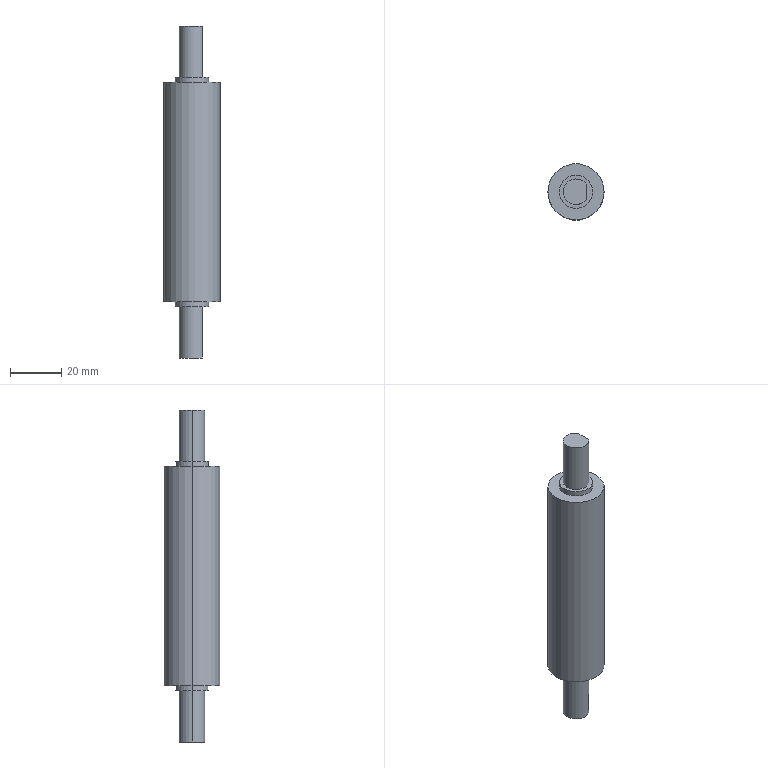Part | STEP file | 08-05 driven shaft | 1 solid | 18 faces | box 22 x 22 x 130 mm | volume 36200 mm3 | cylinder 10 | plane 8 | commonest cylinder face diameters 10 x4 13 x4 22 x2
STEP:
#1=CARTESIAN_POINT('',(-5.,0.,130.));
#2=VERTEX_POINT('',#1);
#3=CARTESIAN_POINT('',(4.,-3.,130.));
#4=VERTEX_POINT('',#3);
#5=CARTESIAN_POINT('',(0.,0.,130.));
#6=DIRECTION('',(0.,0.,1.));
#7=DIRECTION('',(1.,0.,0.));
#8=AXIS2_PLACEMENT_3D('',#5,#6,#7);
#9=CIRCLE('',#8,5.);
#10=EDGE_CURVE('',#2,#4,#9,.T.);
#11=ORIENTED_EDGE('',*,*,#10,.F.);
#12=CARTESIAN_POINT('',(-5.,0.,110.));
#13=VERTEX_POINT('',#12);
#14=CARTESIAN_POINT('',(-5.,0.,130.));
#15=DIRECTION('',(0.,0.,-1.));
#16=VECTOR('',#15,1000.);
#17=LINE('',#14,#16);
#18=EDGE_CURVE('',#2,#13,#17,.T.);
#19=ORIENTED_EDGE('',*,*,#18,.T.);
#20=CARTESIAN_POINT('',(4.,-3.,110.));
#21=VERTEX_POINT('',#20);
#22=CARTESIAN_POINT('',(0.,0.,110.));
#23=DIRECTION('',(0.,0.,1.));
#24=DIRECTION('',(1.,0.,0.));
#25=AXIS2_PLACEMENT_3D('',#22,#23,#24);
#26=CIRCLE('',#25,5.);
#27=EDGE_CURVE('',#13,#21,#26,.T.);
#28=ORIENTED_EDGE('',*,*,#27,.T.);
#29=CARTESIAN_POINT('',(4.,-3.,130.));
#30=DIRECTION('',(0.,0.,1.));
#31=VECTOR('',#30,1000.);
#32=LINE('',#29,#31);
#33=EDGE_CURVE('',#21,#4,#32,.T.);
#34=ORIENTED_EDGE('',*,*,#33,.T.);
#35=EDGE_LOOP('',(#11,#19,#28,#34));
#36=FACE_OUTER_BOUND('',#35,.T.);
#37=CARTESIAN_POINT('',(0.,0.,130.));
#38=DIRECTION('',(0.,0.,-1.));
#39=DIRECTION('',(-1.,0.,0.));
#40=AXIS2_PLACEMENT_3D('',#37,#38,#39);
#41=CYLINDRICAL_SURFACE('',#40,5.);
#42=ADVANCED_FACE('',(#36),#41,.T.);
#43=CARTESIAN_POINT('',(6.5,0.,110.));
#44=VERTEX_POINT('',#43);
#45=CARTESIAN_POINT('',(-6.5,0.,110.));
#46=VERTEX_POINT('',#45);
#47=CARTESIAN_POINT('',(0.,0.,110.));
#48=DIRECTION('',(0.,0.,1.));
#49=DIRECTION('',(1.,0.,0.));
#50=AXIS2_PLACEMENT_3D('',#47,#48,#49);
#51=CIRCLE('',#50,6.5);
#52=EDGE_CURVE('',#44,#46,#51,.T.);
#53=ORIENTED_EDGE('',*,*,#52,.F.);
#54=CARTESIAN_POINT('',(6.5,0.,108.));
#55=VERTEX_POINT('',#54);
#56=CARTESIAN_POINT('',(6.5,0.,110.));
#57=DIRECTION('',(0.,0.,-1.));
#58=VECTOR('',#57,1000.);
#59=LINE('',#56,#58);
#60=EDGE_CURVE('',#44,#55,#59,.T.);
#61=ORIENTED_EDGE('',*,*,#60,.T.);
#62=CARTESIAN_POINT('',(-6.5,0.,108.));
#63=VERTEX_POINT('',#62);
#64=CARTESIAN_POINT('',(0.,0.,108.));
#65=DIRECTION('',(0.,0.,1.));
#66=DIRECTION('',(1.,0.,0.));
#67=AXIS2_PLACEMENT_3D('',#64,#65,#66);
#68=CIRCLE('',#67,6.5);
#69=EDGE_CURVE('',#55,#63,#68,.T.);
#70=ORIENTED_EDGE('',*,*,#69,.T.);
#71=CARTESIAN_POINT('',(-6.5,0.,110.));
#72=DIRECTION('',(0.,0.,-1.));
#73=VECTOR('',#72,1000.);
#74=LINE('',#71,#73);
#75=EDGE_CURVE('',#46,#63,#74,.T.);
#76=ORIENTED_EDGE('',*,*,#75,.F.);
#77=EDGE_LOOP('',(#53,#61,#70,#76));
#78=FACE_OUTER_BOUND('',#77,.T.);
#79=CARTESIAN_POINT('',(0.,0.,110.));
#80=DIRECTION('',(0.,0.,-1.));
#81=DIRECTION('',(-1.,0.,0.));
#82=AXIS2_PLACEMENT_3D('',#79,#80,#81);
#83=CYLINDRICAL_SURFACE('',#82,6.5);
#84=ADVANCED_FACE('',(#78),#83,.T.);
#85=CARTESIAN_POINT('',(4.,-3.,20.));
#86=VERTEX_POINT('',#85);
#87=CARTESIAN_POINT('',(-5.,0.,20.));
#88=VERTEX_POINT('',#87);
#89=CARTESIAN_POINT('',(0.,0.,20.));
#90=DIRECTION('',(0.,0.,-1.));
#91=DIRECTION('',(-1.,0.,0.));
#92=AXIS2_PLACEMENT_3D('',#89,#90,#91);
#93=CIRCLE('',#92,5.);
#94=EDGE_CURVE('',#86,#88,#93,.T.);
#95=ORIENTED_EDGE('',*,*,#94,.T.);
#96=CARTESIAN_POINT('',(-5.,0.,0.));
#97=VERTEX_POINT('',#96);
#98=CARTESIAN_POINT('',(-5.,0.,22.));
#99=DIRECTION('',(0.,0.,-1.));
#100=VECTOR('',#99,1000.);
#101=LINE('',#98,#100);
#102=EDGE_CURVE('',#88,#97,#101,.T.);
#103=ORIENTED_EDGE('',*,*,#102,.T.);
#104=CARTESIAN_POINT('',(4.,-3.,0.));
#105=VERTEX_POINT('',#104);
#106=CARTESIAN_POINT('',(0.,0.,0.));
#107=DIRECTION('',(0.,0.,1.));
#108=DIRECTION('',(1.,0.,0.));
#109=AXIS2_PLACEMENT_3D('',#106,#107,#108);
#110=CIRCLE('',#109,5.);
#111=EDGE_CURVE('',#97,#105,#110,.T.);
#112=ORIENTED_EDGE('',*,*,#111,.T.);
#113=CARTESIAN_POINT('',(4.,-3.,22.));
#114=DIRECTION('',(0.,0.,1.));
#115=VECTOR('',#114,1000.);
#116=LINE('',#113,#115);
#117=EDGE_CURVE('',#105,#86,#116,.T.);
#118=ORIENTED_EDGE('',*,*,#117,.T.);
#119=EDGE_LOOP('',(#95,#103,#112,#118));
#120=FACE_OUTER_BOUND('',#119,.T.);
#121=CARTESIAN_POINT('',(0.,0.,22.));
#122=DIRECTION('',(0.,0.,-1.));
#123=DIRECTION('',(-1.,0.,0.));
#124=AXIS2_PLACEMENT_3D('',#121,#122,#123);
#125=CYLINDRICAL_SURFACE('',#124,5.);
#126=ADVANCED_FACE('',(#120),#125,.T.);
#127=CARTESIAN_POINT('',(-6.5,0.,20.));
#128=VERTEX_POINT('',#127);
#129=CARTESIAN_POINT('',(6.5,0.,20.));
#130=VERTEX_POINT('',#129);
#131=CARTESIAN_POINT('',(0.,0.,20.));
#132=DIRECTION('',(0.,0.,-1.));
#133=DIRECTION('',(-1.,0.,0.));
#134=AXIS2_PLACEMENT_3D('',#131,#132,#133);
#135=CIRCLE('',#134,6.5);
#136=EDGE_CURVE('',#128,#130,#135,.T.);
#137=ORIENTED_EDGE('',*,*,#136,.F.);
#138=CARTESIAN_POINT('',(-6.5,0.,22.));
#139=VERTEX_POINT('',#138);
#140=CARTESIAN_POINT('',(-6.5,0.,20.));
#141=DIRECTION('',(0.,0.,1.));
#142=VECTOR('',#141,1000.);
#143=LINE('',#140,#142);
#144=EDGE_CURVE('',#128,#139,#143,.T.);
#145=ORIENTED_EDGE('',*,*,#144,.T.);
#146=CARTESIAN_POINT('',(6.5,0.,22.));
#147=VERTEX_POINT('',#146);
#148=CARTESIAN_POINT('',(0.,0.,22.));
#149=DIRECTION('',(0.,0.,-1.));
#150=DIRECTION('',(1.,0.,0.));
#151=AXIS2_PLACEMENT_3D('',#148,#149,#150);
#152=CIRCLE('',#151,6.5);
#153=EDGE_CURVE('',#139,#147,#152,.T.);
#154=ORIENTED_EDGE('',*,*,#153,.T.);
#155=CARTESIAN_POINT('',(6.5,0.,20.));
#156=DIRECTION('',(0.,0.,1.));
#157=VECTOR('',#156,1000.);
#158=LINE('',#155,#157);
#159=EDGE_CURVE('',#130,#147,#158,.T.);
#160=ORIENTED_EDGE('',*,*,#159,.F.);
#161=EDGE_LOOP('',(#137,#145,#154,#160));
#162=FACE_OUTER_BOUND('',#161,.T.);
#163=CARTESIAN_POINT('',(0.,0.,20.));
#164=DIRECTION('',(0.,0.,1.));
#165=DIRECTION('',(1.,0.,0.));
#166=AXIS2_PLACEMENT_3D('',#163,#164,#165);
#167=CYLINDRICAL_SURFACE('',#166,6.5);
#168=ADVANCED_FACE('',(#162),#167,.T.);
#169=CARTESIAN_POINT('',(11.,0.,108.));
#170=VERTEX_POINT('',#169);
#171=CARTESIAN_POINT('',(-11.,0.,108.));
#172=VERTEX_POINT('',#171);
#173=CARTESIAN_POINT('',(0.,0.,108.));
#174=DIRECTION('',(0.,0.,1.));
#175=DIRECTION('',(1.,0.,0.));
#176=AXIS2_PLACEMENT_3D('',#173,#174,#175);
#177=CIRCLE('',#176,11.);
#178=EDGE_CURVE('',#170,#172,#177,.T.);
#179=ORIENTED_EDGE('',*,*,#178,.F.);
#180=CARTESIAN_POINT('',(11.,0.,22.));
#181=VERTEX_POINT('',#180);
#182=CARTESIAN_POINT('',(11.,0.,108.));
#183=DIRECTION('',(0.,0.,-1.));
#184=VECTOR('',#183,1000.);
#185=LINE('',#182,#184);
#186=EDGE_CURVE('',#170,#181,#185,.T.);
#187=ORIENTED_EDGE('',*,*,#186,.T.);
#188=CARTESIAN_POINT('',(-11.,0.,22.));
#189=VERTEX_POINT('',#188);
#190=CARTESIAN_POINT('',(0.,0.,22.));
#191=DIRECTION('',(0.,0.,1.));
#192=DIRECTION('',(1.,0.,0.));
#193=AXIS2_PLACEMENT_3D('',#190,#191,#192);
#194=CIRCLE('',#193,11.);
#195=EDGE_CURVE('',#181,#189,#194,.T.);
#196=ORIENTED_EDGE('',*,*,#195,.T.);
#197=CARTESIAN_POINT('',(-11.,0.,108.));
#198=DIRECTION('',(0.,0.,-1.));
#199=VECTOR('',#198,1000.);
#200=LINE('',#197,#199);
#201=EDGE_CURVE('',#172,#189,#200,.T.);
#202=ORIENTED_EDGE('',*,*,#201,.F.);
#203=EDGE_LOOP('',(#179,#187,#196,#202));
#204=FACE_OUTER_BOUND('',#203,.T.);
#205=CARTESIAN_POINT('',(0.,0.,108.));
#206=DIRECTION('',(0.,0.,-1.));
#207=DIRECTION('',(-1.,0.,0.));
#208=AXIS2_PLACEMENT_3D('',#205,#206,#207);
#209=CYLINDRICAL_SURFACE('',#208,11.);
#210=ADVANCED_FACE('',(#204),#209,.T.);
#211=CARTESIAN_POINT('',(4.,3.,110.));
#212=VERTEX_POINT('',#211);
#213=CARTESIAN_POINT('',(0.,0.,110.));
#214=DIRECTION('',(0.,0.,1.));
#215=DIRECTION('',(1.,0.,0.));
#216=AXIS2_PLACEMENT_3D('',#213,#214,#215);
#217=CIRCLE('',#216,5.);
#218=EDGE_CURVE('',#212,#13,#217,.T.);
#219=ORIENTED_EDGE('',*,*,#218,.F.);
#220=CARTESIAN_POINT('',(4.,-5.,110.));
#221=DIRECTION('',(0.,1.,0.));
#222=VECTOR('',#221,1000.);
#223=LINE('',#220,#222);
#224=EDGE_CURVE('',#21,#212,#223,.T.);
#225=ORIENTED_EDGE('',*,*,#224,.F.);
#226=ORIENTED_EDGE('',*,*,#27,.F.);
#227=EDGE_LOOP('',(#219,#225,#226));
#228=FACE_BOUND('',#227,.T.);
#229=CARTESIAN_POINT('',(0.,0.,110.));
#230=DIRECTION('',(0.,0.,1.));
#231=DIRECTION('',(1.,0.,0.));
#232=AXIS2_PLACEMENT_3D('',#229,#230,#231);
#233=CIRCLE('',#232,6.5);
#234=EDGE_CURVE('',#46,#44,#233,.T.);
#235=ORIENTED_EDGE('',*,*,#234,.T.);
#236=ORIENTED_EDGE('',*,*,#52,.T.);
#237=EDGE_LOOP('',(#235,#236));
#238=FACE_OUTER_BOUND('',#237,.T.);
#239=CARTESIAN_POINT('',(0.,0.,110.));
#240=DIRECTION('',(0.,0.,1.));
#241=DIRECTION('',(1.,0.,0.));
#242=AXIS2_PLACEMENT_3D('',#239,#240,#241);
#243=PLANE('',#242);
#244=ADVANCED_FACE('',(#228,#238),#243,.T.);
#245=CARTESIAN_POINT('',(0.,0.,108.));
#246=DIRECTION('',(0.,0.,1.));
#247=DIRECTION('',(1.,0.,0.));
#248=AXIS2_PLACEMENT_3D('',#245,#246,#247);
#249=CIRCLE('',#248,11.);
#250=EDGE_CURVE('',#172,#170,#249,.T.);
#251=ORIENTED_EDGE('',*,*,#250,.T.);
#252=ORIENTED_EDGE('',*,*,#178,.T.);
#253=EDGE_LOOP('',(#251,#252));
#254=FACE_OUTER_BOUND('',#253,.T.);
#255=CARTESIAN_POINT('',(0.,0.,108.));
#256=DIRECTION('',(0.,0.,1.));
#257=DIRECTION('',(1.,0.,0.));
#258=AXIS2_PLACEMENT_3D('',#255,#256,#257);
#259=CIRCLE('',#258,6.5);
#260=EDGE_CURVE('',#63,#55,#259,.T.);
#261=ORIENTED_EDGE('',*,*,#260,.F.);
#262=ORIENTED_EDGE('',*,*,#69,.F.);
#263=EDGE_LOOP('',(#261,#262));
#264=FACE_BOUND('',#263,.T.);
#265=CARTESIAN_POINT('',(0.,0.,108.));
#266=DIRECTION('',(0.,0.,1.));
#267=DIRECTION('',(1.,0.,0.));
#268=AXIS2_PLACEMENT_3D('',#265,#266,#267);
#269=PLANE('',#268);
#270=ADVANCED_FACE('',(#254,#264),#269,.T.);
#271=CARTESIAN_POINT('',(0.,0.,22.));
#272=DIRECTION('',(0.,0.,1.));
#273=DIRECTION('',(1.,0.,0.));
#274=AXIS2_PLACEMENT_3D('',#271,#272,#273);
#275=CIRCLE('',#274,11.);
#276=EDGE_CURVE('',#189,#181,#275,.T.);
#277=ORIENTED_EDGE('',*,*,#276,.F.);
#278=ORIENTED_EDGE('',*,*,#195,.F.);
#279=EDGE_LOOP('',(#277,#278));
#280=FACE_OUTER_BOUND('',#279,.T.);
#281=CARTESIAN_POINT('',(0.,0.,22.));
#282=DIRECTION('',(0.,0.,-1.));
#283=DIRECTION('',(1.,0.,0.));
#284=AXIS2_PLACEMENT_3D('',#281,#282,#283);
#285=CIRCLE('',#284,6.5);
#286=EDGE_CURVE('',#147,#139,#285,.T.);
#287=ORIENTED_EDGE('',*,*,#286,.F.);
#288=ORIENTED_EDGE('',*,*,#153,.F.);
#289=EDGE_LOOP('',(#287,#288));
#290=FACE_BOUND('',#289,.T.);
#291=CARTESIAN_POINT('',(0.,0.,22.));
#292=DIRECTION('',(0.,0.,1.));
#293=DIRECTION('',(1.,0.,0.));
#294=AXIS2_PLACEMENT_3D('',#291,#292,#293);
#295=PLANE('',#294);
#296=ADVANCED_FACE('',(#280,#290),#295,.F.);
#297=ORIENTED_EDGE('',*,*,#186,.F.);
#298=ORIENTED_EDGE('',*,*,#250,.F.);
#299=ORIENTED_EDGE('',*,*,#201,.T.);
#300=ORIENTED_EDGE('',*,*,#276,.T.);
#301=EDGE_LOOP('',(#297,#298,#299,#300));
#302=FACE_OUTER_BOUND('',#301,.T.);
#303=CARTESIAN_POINT('',(0.,0.,108.));
#304=DIRECTION('',(0.,0.,-1.));
#305=DIRECTION('',(-1.,0.,0.));
#306=AXIS2_PLACEMENT_3D('',#303,#304,#305);
#307=CYLINDRICAL_SURFACE('',#306,11.);
#308=ADVANCED_FACE('',(#302),#307,.T.);
#309=ORIENTED_EDGE('',*,*,#94,.F.);
#310=CARTESIAN_POINT('',(4.,3.,20.));
#311=VERTEX_POINT('',#310);
#312=CARTESIAN_POINT('',(4.,-5.,20.));
#313=DIRECTION('',(0.,1.,0.));
#314=VECTOR('',#313,1000.);
#315=LINE('',#312,#314);
#316=EDGE_CURVE('',#86,#311,#315,.T.);
#317=ORIENTED_EDGE('',*,*,#316,.T.);
#318=CARTESIAN_POINT('',(0.,0.,20.));
#319=DIRECTION('',(0.,0.,-1.));
#320=DIRECTION('',(-1.,0.,0.));
#321=AXIS2_PLACEMENT_3D('',#318,#319,#320);
#322=CIRCLE('',#321,5.);
#323=EDGE_CURVE('',#88,#311,#322,.T.);
#324=ORIENTED_EDGE('',*,*,#323,.F.);
#325=EDGE_LOOP('',(#309,#317,#324));
#326=FACE_BOUND('',#325,.T.);
#327=CARTESIAN_POINT('',(0.,0.,20.));
#328=DIRECTION('',(0.,0.,-1.));
#329=DIRECTION('',(-1.,0.,0.));
#330=AXIS2_PLACEMENT_3D('',#327,#328,#329);
#331=CIRCLE('',#330,6.5);
#332=EDGE_CURVE('',#130,#128,#331,.T.);
#333=ORIENTED_EDGE('',*,*,#332,.T.);
#334=ORIENTED_EDGE('',*,*,#136,.T.);
#335=EDGE_LOOP('',(#333,#334));
#336=FACE_OUTER_BOUND('',#335,.T.);
#337=CARTESIAN_POINT('',(0.,0.,20.));
#338=DIRECTION('',(0.,0.,-1.));
#339=DIRECTION('',(-1.,0.,0.));
#340=AXIS2_PLACEMENT_3D('',#337,#338,#339);
#341=PLANE('',#340);
#342=ADVANCED_FACE('',(#326,#336),#341,.T.);
#343=ORIENTED_EDGE('',*,*,#144,.F.);
#344=ORIENTED_EDGE('',*,*,#332,.F.);
#345=ORIENTED_EDGE('',*,*,#159,.T.);
#346=ORIENTED_EDGE('',*,*,#286,.T.);
#347=EDGE_LOOP('',(#343,#344,#345,#346));
#348=FACE_OUTER_BOUND('',#347,.T.);
#349=CARTESIAN_POINT('',(0.,0.,20.));
#350=DIRECTION('',(0.,0.,1.));
#351=DIRECTION('',(1.,0.,0.));
#352=AXIS2_PLACEMENT_3D('',#349,#350,#351);
#353=CYLINDRICAL_SURFACE('',#352,6.5);
#354=ADVANCED_FACE('',(#348),#353,.T.);
#355=CARTESIAN_POINT('',(4.,3.,0.));
#356=VERTEX_POINT('',#355);
#357=CARTESIAN_POINT('',(0.,0.,0.));
#358=DIRECTION('',(0.,0.,1.));
#359=DIRECTION('',(1.,0.,0.));
#360=AXIS2_PLACEMENT_3D('',#357,#358,#359);
#361=CIRCLE('',#360,5.);
#362=EDGE_CURVE('',#356,#97,#361,.T.);
#363=ORIENTED_EDGE('',*,*,#362,.F.);
#364=CARTESIAN_POINT('',(4.,0.,0.));
#365=DIRECTION('',(0.,-1.,0.));
#366=VECTOR('',#365,1000.);
#367=LINE('',#364,#366);
#368=EDGE_CURVE('',#356,#105,#367,.T.);
#369=ORIENTED_EDGE('',*,*,#368,.T.);
#370=ORIENTED_EDGE('',*,*,#111,.F.);
#371=EDGE_LOOP('',(#363,#369,#370));
#372=FACE_OUTER_BOUND('',#371,.T.);
#373=CARTESIAN_POINT('',(0.,0.,0.));
#374=DIRECTION('',(0.,0.,1.));
#375=DIRECTION('',(1.,0.,0.));
#376=AXIS2_PLACEMENT_3D('',#373,#374,#375);
#377=PLANE('',#376);
#378=ADVANCED_FACE('',(#372),#377,.F.);
#379=ORIENTED_EDGE('',*,*,#102,.F.);
#380=ORIENTED_EDGE('',*,*,#323,.T.);
#381=CARTESIAN_POINT('',(4.,3.,22.));
#382=DIRECTION('',(0.,0.,-1.));
#383=VECTOR('',#382,1000.);
#384=LINE('',#381,#383);
#385=EDGE_CURVE('',#311,#356,#384,.T.);
#386=ORIENTED_EDGE('',*,*,#385,.T.);
#387=ORIENTED_EDGE('',*,*,#362,.T.);
#388=EDGE_LOOP('',(#379,#380,#386,#387));
#389=FACE_OUTER_BOUND('',#388,.T.);
#390=CARTESIAN_POINT('',(0.,0.,22.));
#391=DIRECTION('',(0.,0.,-1.));
#392=DIRECTION('',(-1.,0.,0.));
#393=AXIS2_PLACEMENT_3D('',#390,#391,#392);
#394=CYLINDRICAL_SURFACE('',#393,5.);
#395=ADVANCED_FACE('',(#389),#394,.T.);
#396=ORIENTED_EDGE('',*,*,#60,.F.);
#397=ORIENTED_EDGE('',*,*,#234,.F.);
#398=ORIENTED_EDGE('',*,*,#75,.T.);
#399=ORIENTED_EDGE('',*,*,#260,.T.);
#400=EDGE_LOOP('',(#396,#397,#398,#399));
#401=FACE_OUTER_BOUND('',#400,.T.);
#402=CARTESIAN_POINT('',(0.,0.,110.));
#403=DIRECTION('',(0.,0.,-1.));
#404=DIRECTION('',(-1.,0.,0.));
#405=AXIS2_PLACEMENT_3D('',#402,#403,#404);
#406=CYLINDRICAL_SURFACE('',#405,6.5);
#407=ADVANCED_FACE('',(#401),#406,.T.);
#408=ORIENTED_EDGE('',*,*,#18,.F.);
#409=CARTESIAN_POINT('',(4.,3.,130.));
#410=VERTEX_POINT('',#409);
#411=CARTESIAN_POINT('',(0.,0.,130.));
#412=DIRECTION('',(0.,0.,1.));
#413=DIRECTION('',(1.,0.,0.));
#414=AXIS2_PLACEMENT_3D('',#411,#412,#413);
#415=CIRCLE('',#414,5.);
#416=EDGE_CURVE('',#410,#2,#415,.T.);
#417=ORIENTED_EDGE('',*,*,#416,.F.);
#418=CARTESIAN_POINT('',(4.,3.,130.));
#419=DIRECTION('',(0.,0.,-1.));
#420=VECTOR('',#419,1000.);
#421=LINE('',#418,#420);
#422=EDGE_CURVE('',#410,#212,#421,.T.);
#423=ORIENTED_EDGE('',*,*,#422,.T.);
#424=ORIENTED_EDGE('',*,*,#218,.T.);
#425=EDGE_LOOP('',(#408,#417,#423,#424));
#426=FACE_OUTER_BOUND('',#425,.T.);
#427=CARTESIAN_POINT('',(0.,0.,130.));
#428=DIRECTION('',(0.,0.,-1.));
#429=DIRECTION('',(-1.,0.,0.));
#430=AXIS2_PLACEMENT_3D('',#427,#428,#429);
#431=CYLINDRICAL_SURFACE('',#430,5.);
#432=ADVANCED_FACE('',(#426),#431,.T.);
#433=CARTESIAN_POINT('',(4.,0.,130.));
#434=DIRECTION('',(0.,-1.,0.));
#435=VECTOR('',#434,1000.);
#436=LINE('',#433,#435);
#437=EDGE_CURVE('',#410,#4,#436,.T.);
#438=ORIENTED_EDGE('',*,*,#437,.F.);
#439=ORIENTED_EDGE('',*,*,#416,.T.);
#440=ORIENTED_EDGE('',*,*,#10,.T.);
#441=EDGE_LOOP('',(#438,#439,#440));
#442=FACE_OUTER_BOUND('',#441,.T.);
#443=CARTESIAN_POINT('',(0.,0.,130.));
#444=DIRECTION('',(0.,0.,1.));
#445=DIRECTION('',(1.,0.,0.));
#446=AXIS2_PLACEMENT_3D('',#443,#444,#445);
#447=PLANE('',#446);
#448=ADVANCED_FACE('',(#442),#447,.T.);
#449=ORIENTED_EDGE('',*,*,#316,.F.);
#450=ORIENTED_EDGE('',*,*,#117,.F.);
#451=ORIENTED_EDGE('',*,*,#368,.F.);
#452=ORIENTED_EDGE('',*,*,#385,.F.);
#453=EDGE_LOOP('',(#449,#450,#451,#452));
#454=FACE_OUTER_BOUND('',#453,.T.);
#455=CARTESIAN_POINT('',(4.,-5.,20.));
#456=DIRECTION('',(-1.,0.,0.));
#457=DIRECTION('',(0.,0.,1.));
#458=AXIS2_PLACEMENT_3D('',#455,#456,#457);
#459=PLANE('',#458);
#460=ADVANCED_FACE('',(#454),#459,.F.);
#461=ORIENTED_EDGE('',*,*,#437,.T.);
#462=ORIENTED_EDGE('',*,*,#33,.F.);
#463=ORIENTED_EDGE('',*,*,#224,.T.);
#464=ORIENTED_EDGE('',*,*,#422,.F.);
#465=EDGE_LOOP('',(#461,#462,#463,#464));
#466=FACE_OUTER_BOUND('',#465,.T.);
#467=CARTESIAN_POINT('',(4.,-5.,110.));
#468=DIRECTION('',(-1.,0.,0.));
#469=DIRECTION('',(0.,0.,1.));
#470=AXIS2_PLACEMENT_3D('',#467,#468,#469);
#471=PLANE('',#470);
#472=ADVANCED_FACE('',(#466),#471,.F.);
#473=CLOSED_SHELL('',(#42,#84,#126,#168,#210,#244,#270,#296,#308,#342,#354,#378,#395,#407,#432,#448,#460,#472));
#474=MANIFOLD_SOLID_BREP('',#473);
#475=CARTESIAN_POINT('',(0.,0.,0.));
#476=DIRECTION('',(0.,0.,1.));
#477=DIRECTION('',(1.,0.,0.));
#478=AXIS2_PLACEMENT_3D('',#475,#476,#477);
#479=(LENGTH_UNIT()NAMED_UNIT(*)SI_UNIT(.MILLI.,.METRE.));
#480=UNCERTAINTY_MEASURE_WITH_UNIT(LENGTH_MEASURE(0.00001),#479,'','');
#481=(NAMED_UNIT(*)PLANE_ANGLE_UNIT()SI_UNIT($,.RADIAN.));
#482=(NAMED_UNIT(*)SI_UNIT($,.STERADIAN.)SOLID_ANGLE_UNIT());
#483=(GEOMETRIC_REPRESENTATION_CONTEXT(3)GLOBAL_UNCERTAINTY_ASSIGNED_CONTEXT((#480))GLOBAL_UNIT_ASSIGNED_CONTEXT((#479,#481,#482))REPRESENTATION_CONTEXT('',''));
#484=ADVANCED_BREP_SHAPE_REPRESENTATION('',(#474,#478),#483);